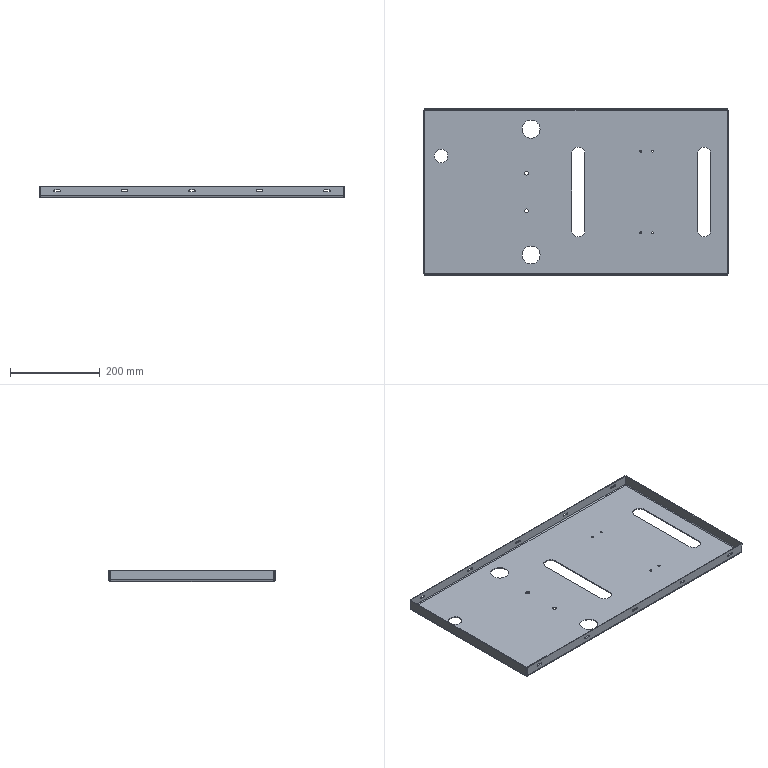Part | SolidWorks | features ICE 4, Cut 1, EdgeFlange 1, FlatPattern 1, HoleWzd 1, SMBaseFlange 1, SheetMetal 1 | 1 solid | 104 faces | box 680 x 370 x 25 mm | volume 562100 mm3 | cylinder 50 | plane 46 | spline 8 | commonest cylinder face diameters 4.5 x20 4.8 x8 30 x6 4 x4 8 x4 8.5 x4